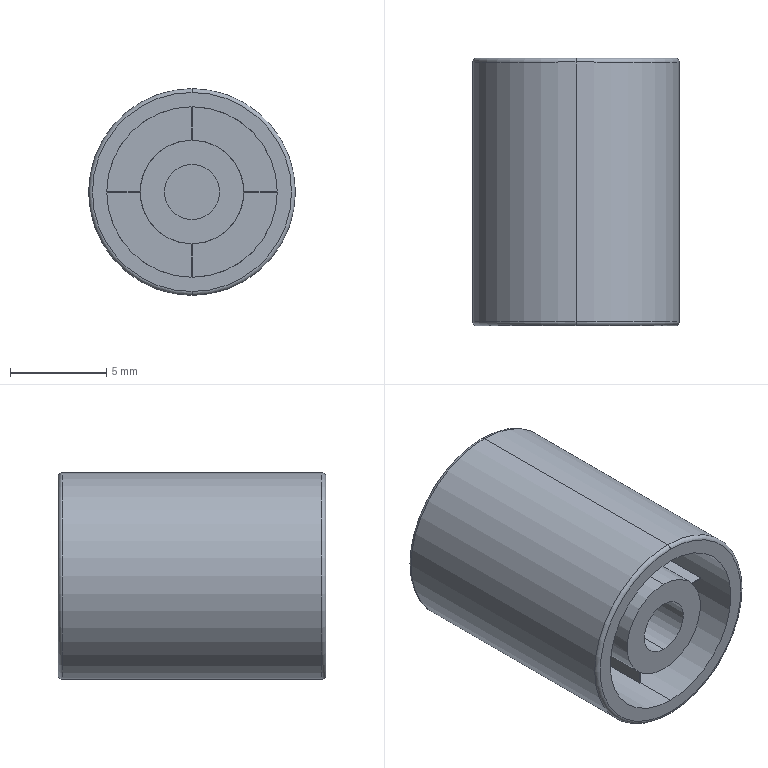Part | SolidWorks | features BaseBody 1 | 1 solid | 60 faces | box 10.75 x 13.9 x 10.75 mm | volume 660.288 mm3 | plane 38 | cylinder 14 | torus 8 | commonest cylinder face diameters 2.87 x4 5.39 x4 8.87 x4 10.75 x2